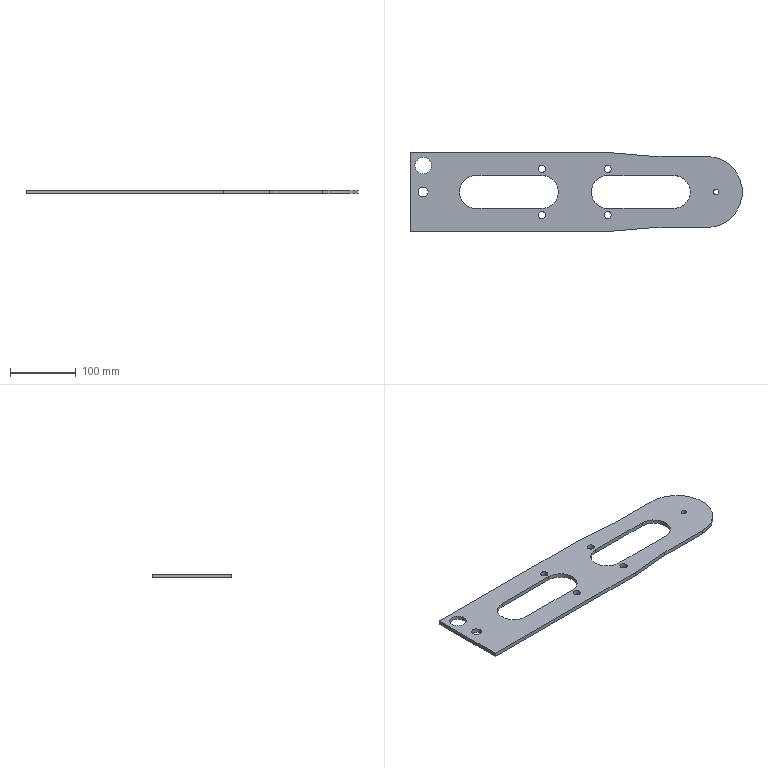Part | SolidWorks | features Extrusion 1, HoleWzd 1, ICE 1 | 1 solid | 34 faces | box 504 x 120 x 6 mm | volume 253053 mm3 | cylinder 21 | plane 13 | commonest cylinder face diameters 11 x8 50 x6 8 x2 15 x2 25 x2 108 x1
STEP:
#1=CARTESIAN_POINT('',(205.5,60.,6.));
#2=VERTEX_POINT('',#1);
#3=CARTESIAN_POINT('',(213.5,60.,6.));
#4=VERTEX_POINT('',#3);
#5=CARTESIAN_POINT('',(209.5,60.,6.));
#6=DIRECTION('',(0.,0.,1.));
#7=DIRECTION('',(1.,0.,0.));
#8=AXIS2_PLACEMENT_3D('',#5,#6,#7);
#9=CIRCLE('',#8,4.);
#10=EDGE_CURVE('',#2,#4,#9,.T.);
#11=ORIENTED_EDGE('',*,*,#10,.T.);
#12=CARTESIAN_POINT('',(213.5,60.,0.));
#13=VERTEX_POINT('',#12);
#14=CARTESIAN_POINT('',(213.5,60.,10.));
#15=DIRECTION('',(0.,0.,-1.));
#16=VECTOR('',#15,1000.);
#17=LINE('',#14,#16);
#18=EDGE_CURVE('',#4,#13,#17,.T.);
#19=ORIENTED_EDGE('',*,*,#18,.T.);
#20=CARTESIAN_POINT('',(205.5,60.,0.));
#21=VERTEX_POINT('',#20);
#22=CARTESIAN_POINT('',(209.5,60.,0.));
#23=DIRECTION('',(0.,0.,-1.));
#24=DIRECTION('',(-1.,0.,0.));
#25=AXIS2_PLACEMENT_3D('',#22,#23,#24);
#26=CIRCLE('',#25,4.);
#27=EDGE_CURVE('',#13,#21,#26,.T.);
#28=ORIENTED_EDGE('',*,*,#27,.T.);
#29=CARTESIAN_POINT('',(205.5,60.,10.));
#30=DIRECTION('',(0.,0.,-1.));
#31=VECTOR('',#30,1000.);
#32=LINE('',#29,#31);
#33=EDGE_CURVE('',#2,#21,#32,.T.);
#34=ORIENTED_EDGE('',*,*,#33,.F.);
#35=EDGE_LOOP('',(#11,#19,#28,#34));
#36=FACE_OUTER_BOUND('',#35,.T.);
#37=CARTESIAN_POINT('',(209.5,60.,10.));
#38=DIRECTION('',(0.,0.,-1.));
#39=DIRECTION('',(-1.,0.,0.));
#40=AXIS2_PLACEMENT_3D('',#37,#38,#39);
#41=CYLINDRICAL_SURFACE('',#40,4.);
#42=ADVANCED_FACE('',(#36),#41,.F.);
#43=CARTESIAN_POINT('',(-60.5,95.,0.));
#44=VERTEX_POINT('',#43);
#45=CARTESIAN_POINT('',(-49.5,95.,0.));
#46=VERTEX_POINT('',#45);
#47=CARTESIAN_POINT('',(-55.,95.,0.));
#48=DIRECTION('',(0.,0.,1.));
#49=DIRECTION('',(1.,0.,0.));
#50=AXIS2_PLACEMENT_3D('',#47,#48,#49);
#51=CIRCLE('',#50,5.5);
#52=EDGE_CURVE('',#44,#46,#51,.T.);
#53=ORIENTED_EDGE('',*,*,#52,.F.);
#54=CARTESIAN_POINT('',(-60.5,95.,6.));
#55=VERTEX_POINT('',#54);
#56=CARTESIAN_POINT('',(-60.5,95.,6.));
#57=DIRECTION('',(0.,0.,1.));
#58=VECTOR('',#57,1000.);
#59=LINE('',#56,#58);
#60=EDGE_CURVE('',#44,#55,#59,.T.);
#61=ORIENTED_EDGE('',*,*,#60,.T.);
#62=CARTESIAN_POINT('',(-49.5,95.,6.));
#63=VERTEX_POINT('',#62);
#64=CARTESIAN_POINT('',(-55.,95.,6.));
#65=DIRECTION('',(0.,0.,1.));
#66=DIRECTION('',(1.,0.,0.));
#67=AXIS2_PLACEMENT_3D('',#64,#65,#66);
#68=CIRCLE('',#67,5.5);
#69=EDGE_CURVE('',#55,#63,#68,.T.);
#70=ORIENTED_EDGE('',*,*,#69,.T.);
#71=CARTESIAN_POINT('',(-49.5,95.,6.));
#72=DIRECTION('',(0.,0.,1.));
#73=VECTOR('',#72,1000.);
#74=LINE('',#71,#73);
#75=EDGE_CURVE('',#46,#63,#74,.T.);
#76=ORIENTED_EDGE('',*,*,#75,.F.);
#77=EDGE_LOOP('',(#53,#61,#70,#76));
#78=FACE_OUTER_BOUND('',#77,.T.);
#79=CARTESIAN_POINT('',(-55.,95.,6.));
#80=DIRECTION('',(0.,0.,1.));
#81=DIRECTION('',(1.,0.,0.));
#82=AXIS2_PLACEMENT_3D('',#79,#80,#81);
#83=CYLINDRICAL_SURFACE('',#82,5.5);
#84=ADVANCED_FACE('',(#78),#83,.F.);
#85=CARTESIAN_POINT('',(-60.5,25.,0.));
#86=VERTEX_POINT('',#85);
#87=CARTESIAN_POINT('',(-49.5,25.,0.));
#88=VERTEX_POINT('',#87);
#89=CARTESIAN_POINT('',(-55.,25.,0.));
#90=DIRECTION('',(0.,0.,1.));
#91=DIRECTION('',(1.,0.,0.));
#92=AXIS2_PLACEMENT_3D('',#89,#90,#91);
#93=CIRCLE('',#92,5.5);
#94=EDGE_CURVE('',#86,#88,#93,.T.);
#95=ORIENTED_EDGE('',*,*,#94,.F.);
#96=CARTESIAN_POINT('',(-60.5,25.,6.));
#97=VERTEX_POINT('',#96);
#98=CARTESIAN_POINT('',(-60.5,25.,6.));
#99=DIRECTION('',(0.,0.,1.));
#100=VECTOR('',#99,1000.);
#101=LINE('',#98,#100);
#102=EDGE_CURVE('',#86,#97,#101,.T.);
#103=ORIENTED_EDGE('',*,*,#102,.T.);
#104=CARTESIAN_POINT('',(-49.5,25.,6.));
#105=VERTEX_POINT('',#104);
#106=CARTESIAN_POINT('',(-55.,25.,6.));
#107=DIRECTION('',(0.,0.,1.));
#108=DIRECTION('',(1.,0.,0.));
#109=AXIS2_PLACEMENT_3D('',#106,#107,#108);
#110=CIRCLE('',#109,5.5);
#111=EDGE_CURVE('',#97,#105,#110,.T.);
#112=ORIENTED_EDGE('',*,*,#111,.T.);
#113=CARTESIAN_POINT('',(-49.5,25.,6.));
#114=DIRECTION('',(0.,0.,1.));
#115=VECTOR('',#114,1000.);
#116=LINE('',#113,#115);
#117=EDGE_CURVE('',#88,#105,#116,.T.);
#118=ORIENTED_EDGE('',*,*,#117,.F.);
#119=EDGE_LOOP('',(#95,#103,#112,#118));
#120=FACE_OUTER_BOUND('',#119,.T.);
#121=CARTESIAN_POINT('',(-55.,25.,6.));
#122=DIRECTION('',(0.,0.,1.));
#123=DIRECTION('',(1.,0.,0.));
#124=AXIS2_PLACEMENT_3D('',#121,#122,#123);
#125=CYLINDRICAL_SURFACE('',#124,5.5);
#126=ADVANCED_FACE('',(#120),#125,.F.);
#127=CARTESIAN_POINT('',(39.5,95.,0.));
#128=VERTEX_POINT('',#127);
#129=CARTESIAN_POINT('',(50.5,95.,0.));
#130=VERTEX_POINT('',#129);
#131=CARTESIAN_POINT('',(45.,95.,0.));
#132=DIRECTION('',(0.,0.,1.));
#133=DIRECTION('',(1.,0.,0.));
#134=AXIS2_PLACEMENT_3D('',#131,#132,#133);
#135=CIRCLE('',#134,5.5);
#136=EDGE_CURVE('',#128,#130,#135,.T.);
#137=ORIENTED_EDGE('',*,*,#136,.F.);
#138=CARTESIAN_POINT('',(39.5,95.,6.));
#139=VERTEX_POINT('',#138);
#140=CARTESIAN_POINT('',(39.5,95.,6.));
#141=DIRECTION('',(0.,0.,1.));
#142=VECTOR('',#141,1000.);
#143=LINE('',#140,#142);
#144=EDGE_CURVE('',#128,#139,#143,.T.);
#145=ORIENTED_EDGE('',*,*,#144,.T.);
#146=CARTESIAN_POINT('',(50.5,95.,6.));
#147=VERTEX_POINT('',#146);
#148=CARTESIAN_POINT('',(45.,95.,6.));
#149=DIRECTION('',(0.,0.,1.));
#150=DIRECTION('',(1.,0.,0.));
#151=AXIS2_PLACEMENT_3D('',#148,#149,#150);
#152=CIRCLE('',#151,5.5);
#153=EDGE_CURVE('',#139,#147,#152,.T.);
#154=ORIENTED_EDGE('',*,*,#153,.T.);
#155=CARTESIAN_POINT('',(50.5,95.,6.));
#156=DIRECTION('',(0.,0.,1.));
#157=VECTOR('',#156,1000.);
#158=LINE('',#155,#157);
#159=EDGE_CURVE('',#130,#147,#158,.T.);
#160=ORIENTED_EDGE('',*,*,#159,.F.);
#161=EDGE_LOOP('',(#137,#145,#154,#160));
#162=FACE_OUTER_BOUND('',#161,.T.);
#163=CARTESIAN_POINT('',(45.,95.,6.));
#164=DIRECTION('',(0.,0.,1.));
#165=DIRECTION('',(1.,0.,0.));
#166=AXIS2_PLACEMENT_3D('',#163,#164,#165);
#167=CYLINDRICAL_SURFACE('',#166,5.5);
#168=ADVANCED_FACE('',(#162),#167,.F.);
#169=CARTESIAN_POINT('',(39.5,25.,0.));
#170=VERTEX_POINT('',#169);
#171=CARTESIAN_POINT('',(50.5,25.,0.));
#172=VERTEX_POINT('',#171);
#173=CARTESIAN_POINT('',(45.,25.,0.));
#174=DIRECTION('',(0.,0.,1.));
#175=DIRECTION('',(1.,0.,0.));
#176=AXIS2_PLACEMENT_3D('',#173,#174,#175);
#177=CIRCLE('',#176,5.5);
#178=EDGE_CURVE('',#170,#172,#177,.T.);
#179=ORIENTED_EDGE('',*,*,#178,.F.);
#180=CARTESIAN_POINT('',(39.5,25.,6.));
#181=VERTEX_POINT('',#180);
#182=CARTESIAN_POINT('',(39.5,25.,6.));
#183=DIRECTION('',(0.,0.,1.));
#184=VECTOR('',#183,1000.);
#185=LINE('',#182,#184);
#186=EDGE_CURVE('',#170,#181,#185,.T.);
#187=ORIENTED_EDGE('',*,*,#186,.T.);
#188=CARTESIAN_POINT('',(50.5,25.,6.));
#189=VERTEX_POINT('',#188);
#190=CARTESIAN_POINT('',(45.,25.,6.));
#191=DIRECTION('',(0.,0.,1.));
#192=DIRECTION('',(1.,0.,0.));
#193=AXIS2_PLACEMENT_3D('',#190,#191,#192);
#194=CIRCLE('',#193,5.5);
#195=EDGE_CURVE('',#181,#189,#194,.T.);
#196=ORIENTED_EDGE('',*,*,#195,.T.);
#197=CARTESIAN_POINT('',(50.5,25.,6.));
#198=DIRECTION('',(0.,0.,1.));
#199=VECTOR('',#198,1000.);
#200=LINE('',#197,#199);
#201=EDGE_CURVE('',#172,#189,#200,.T.);
#202=ORIENTED_EDGE('',*,*,#201,.F.);
#203=EDGE_LOOP('',(#179,#187,#196,#202));
#204=FACE_OUTER_BOUND('',#203,.T.);
#205=CARTESIAN_POINT('',(45.,25.,6.));
#206=DIRECTION('',(0.,0.,1.));
#207=DIRECTION('',(1.,0.,0.));
#208=AXIS2_PLACEMENT_3D('',#205,#206,#207);
#209=CYLINDRICAL_SURFACE('',#208,5.5);
#210=ADVANCED_FACE('',(#204),#209,.F.);
#211=CARTESIAN_POINT('',(45.,85.,6.));
#212=VERTEX_POINT('',#211);
#213=CARTESIAN_POINT('',(20.,60.,6.));
#214=VERTEX_POINT('',#213);
#215=CARTESIAN_POINT('',(45.,60.,6.));
#216=DIRECTION('',(0.,0.,1.));
#217=DIRECTION('',(1.,0.,0.));
#218=AXIS2_PLACEMENT_3D('',#215,#216,#217);
#219=CIRCLE('',#218,25.);
#220=EDGE_CURVE('',#212,#214,#219,.T.);
#221=ORIENTED_EDGE('',*,*,#220,.T.);
#222=CARTESIAN_POINT('',(20.,60.,0.));
#223=VERTEX_POINT('',#222);
#224=CARTESIAN_POINT('',(20.,60.,6.));
#225=DIRECTION('',(0.,0.,-1.));
#226=VECTOR('',#225,1000.);
#227=LINE('',#224,#226);
#228=EDGE_CURVE('',#214,#223,#227,.T.);
#229=ORIENTED_EDGE('',*,*,#228,.T.);
#230=CARTESIAN_POINT('',(45.,85.,0.));
#231=VERTEX_POINT('',#230);
#232=CARTESIAN_POINT('',(45.,60.,0.));
#233=DIRECTION('',(0.,0.,1.));
#234=DIRECTION('',(1.,0.,0.));
#235=AXIS2_PLACEMENT_3D('',#232,#233,#234);
#236=CIRCLE('',#235,25.);
#237=EDGE_CURVE('',#231,#223,#236,.T.);
#238=ORIENTED_EDGE('',*,*,#237,.F.);
#239=CARTESIAN_POINT('',(45.,85.,6.));
#240=DIRECTION('',(0.,0.,-1.));
#241=VECTOR('',#240,1000.);
#242=LINE('',#239,#241);
#243=EDGE_CURVE('',#212,#231,#242,.T.);
#244=ORIENTED_EDGE('',*,*,#243,.F.);
#245=EDGE_LOOP('',(#221,#229,#238,#244));
#246=FACE_OUTER_BOUND('',#245,.T.);
#247=CARTESIAN_POINT('',(45.,60.,6.));
#248=DIRECTION('',(0.,0.,-1.));
#249=DIRECTION('',(-1.,0.,0.));
#250=AXIS2_PLACEMENT_3D('',#247,#248,#249);
#251=CYLINDRICAL_SURFACE('',#250,25.);
#252=ADVANCED_FACE('',(#246),#251,.F.);
#253=CARTESIAN_POINT('',(-155.,85.,6.));
#254=VERTEX_POINT('',#253);
#255=CARTESIAN_POINT('',(-180.,60.,6.));
#256=VERTEX_POINT('',#255);
#257=CARTESIAN_POINT('',(-155.,60.,6.));
#258=DIRECTION('',(0.,0.,1.));
#259=DIRECTION('',(1.,0.,0.));
#260=AXIS2_PLACEMENT_3D('',#257,#258,#259);
#261=CIRCLE('',#260,25.);
#262=EDGE_CURVE('',#254,#256,#261,.T.);
#263=ORIENTED_EDGE('',*,*,#262,.T.);
#264=CARTESIAN_POINT('',(-180.,60.,0.));
#265=VERTEX_POINT('',#264);
#266=CARTESIAN_POINT('',(-180.,60.,6.));
#267=DIRECTION('',(0.,0.,-1.));
#268=VECTOR('',#267,1000.);
#269=LINE('',#266,#268);
#270=EDGE_CURVE('',#256,#265,#269,.T.);
#271=ORIENTED_EDGE('',*,*,#270,.T.);
#272=CARTESIAN_POINT('',(-155.,85.,0.));
#273=VERTEX_POINT('',#272);
#274=CARTESIAN_POINT('',(-155.,60.,0.));
#275=DIRECTION('',(0.,0.,1.));
#276=DIRECTION('',(1.,0.,0.));
#277=AXIS2_PLACEMENT_3D('',#274,#275,#276);
#278=CIRCLE('',#277,25.);
#279=EDGE_CURVE('',#273,#265,#278,.T.);
#280=ORIENTED_EDGE('',*,*,#279,.F.);
#281=CARTESIAN_POINT('',(-155.,85.,6.));
#282=DIRECTION('',(0.,0.,-1.));
#283=VECTOR('',#282,1000.);
#284=LINE('',#281,#283);
#285=EDGE_CURVE('',#254,#273,#284,.T.);
#286=ORIENTED_EDGE('',*,*,#285,.F.);
#287=EDGE_LOOP('',(#263,#271,#280,#286));
#288=FACE_OUTER_BOUND('',#287,.T.);
#289=CARTESIAN_POINT('',(-155.,60.,6.));
#290=DIRECTION('',(0.,0.,-1.));
#291=DIRECTION('',(-1.,0.,0.));
#292=AXIS2_PLACEMENT_3D('',#289,#290,#291);
#293=CYLINDRICAL_SURFACE('',#292,25.);
#294=ADVANCED_FACE('',(#288),#293,.F.);
#295=CARTESIAN_POINT('',(-242.5,60.,6.));
#296=VERTEX_POINT('',#295);
#297=CARTESIAN_POINT('',(-227.5,60.,6.));
#298=VERTEX_POINT('',#297);
#299=CARTESIAN_POINT('',(-235.,60.,6.));
#300=DIRECTION('',(0.,0.,1.));
#301=DIRECTION('',(1.,0.,0.));
#302=AXIS2_PLACEMENT_3D('',#299,#300,#301);
#303=CIRCLE('',#302,7.5);
#304=EDGE_CURVE('',#296,#298,#303,.T.);
#305=ORIENTED_EDGE('',*,*,#304,.T.);
#306=CARTESIAN_POINT('',(-227.5,60.,0.));
#307=VERTEX_POINT('',#306);
#308=CARTESIAN_POINT('',(-227.5,60.,6.));
#309=DIRECTION('',(0.,0.,-1.));
#310=VECTOR('',#309,1000.);
#311=LINE('',#308,#310);
#312=EDGE_CURVE('',#298,#307,#311,.T.);
#313=ORIENTED_EDGE('',*,*,#312,.T.);
#314=CARTESIAN_POINT('',(-242.5,60.,0.));
#315=VERTEX_POINT('',#314);
#316=CARTESIAN_POINT('',(-235.,60.,0.));
#317=DIRECTION('',(0.,0.,1.));
#318=DIRECTION('',(1.,0.,0.));
#319=AXIS2_PLACEMENT_3D('',#316,#317,#318);
#320=CIRCLE('',#319,7.5);
#321=EDGE_CURVE('',#315,#307,#320,.T.);
#322=ORIENTED_EDGE('',*,*,#321,.F.);
#323=CARTESIAN_POINT('',(-242.5,60.,6.));
#324=DIRECTION('',(0.,0.,-1.));
#325=VECTOR('',#324,1000.);
#326=LINE('',#323,#325);
#327=EDGE_CURVE('',#296,#315,#326,.T.);
#328=ORIENTED_EDGE('',*,*,#327,.F.);
#329=EDGE_LOOP('',(#305,#313,#322,#328));
#330=FACE_OUTER_BOUND('',#329,.T.);
#331=CARTESIAN_POINT('',(-235.,60.,6.));
#332=DIRECTION('',(0.,0.,-1.));
#333=DIRECTION('',(-1.,0.,0.));
#334=AXIS2_PLACEMENT_3D('',#331,#332,#333);
#335=CYLINDRICAL_SURFACE('',#334,7.5);
#336=ADVANCED_FACE('',(#330),#335,.F.);
#337=CARTESIAN_POINT('',(-247.5,100.,6.));
#338=VERTEX_POINT('',#337);
#339=CARTESIAN_POINT('',(-222.5,100.,6.));
#340=VERTEX_POINT('',#339);
#341=CARTESIAN_POINT('',(-235.,100.,6.));
#342=DIRECTION('',(0.,0.,1.));
#343=DIRECTION('',(1.,0.,0.));
#344=AXIS2_PLACEMENT_3D('',#341,#342,#343);
#345=CIRCLE('',#344,12.5);
#346=EDGE_CURVE('',#338,#340,#345,.T.);
#347=ORIENTED_EDGE('',*,*,#346,.T.);
#348=CARTESIAN_POINT('',(-222.5,100.,0.));
#349=VERTEX_POINT('',#348);
#350=CARTESIAN_POINT('',(-222.5,100.,6.));
#351=DIRECTION('',(0.,0.,-1.));
#352=VECTOR('',#351,1000.);
#353=LINE('',#350,#352);
#354=EDGE_CURVE('',#340,#349,#353,.T.);
#355=ORIENTED_EDGE('',*,*,#354,.T.);
#356=CARTESIAN_POINT('',(-247.5,100.,0.));
#357=VERTEX_POINT('',#356);
#358=CARTESIAN_POINT('',(-235.,100.,0.));
#359=DIRECTION('',(0.,0.,1.));
#360=DIRECTION('',(1.,0.,0.));
#361=AXIS2_PLACEMENT_3D('',#358,#359,#360);
#362=CIRCLE('',#361,12.5);
#363=EDGE_CURVE('',#357,#349,#362,.T.);
#364=ORIENTED_EDGE('',*,*,#363,.F.);
#365=CARTESIAN_POINT('',(-247.5,100.,6.));
#366=DIRECTION('',(0.,0.,-1.));
#367=VECTOR('',#366,1000.);
#368=LINE('',#365,#367);
#369=EDGE_CURVE('',#338,#357,#368,.T.);
#370=ORIENTED_EDGE('',*,*,#369,.F.);
#371=EDGE_LOOP('',(#347,#355,#364,#370));
#372=FACE_OUTER_BOUND('',#371,.T.);
#373=CARTESIAN_POINT('',(-235.,100.,6.));
#374=DIRECTION('',(0.,0.,-1.));
#375=DIRECTION('',(-1.,0.,0.));
#376=AXIS2_PLACEMENT_3D('',#373,#374,#375);
#377=CYLINDRICAL_SURFACE('',#376,12.5);
#378=ADVANCED_FACE('',(#372),#377,.F.);
#379=CARTESIAN_POINT('',(209.5,60.,0.));
#380=DIRECTION('',(0.,0.,-1.));
#381=DIRECTION('',(-1.,0.,0.));
#382=AXIS2_PLACEMENT_3D('',#379,#380,#381);
#383=CIRCLE('',#382,4.);
#384=EDGE_CURVE('',#21,#13,#383,.T.);
#385=ORIENTED_EDGE('',*,*,#384,.F.);
#386=ORIENTED_EDGE('',*,*,#27,.F.);
#387=EDGE_LOOP('',(#385,#386));
#388=FACE_BOUND('',#387,.T.);
#389=CARTESIAN_POINT('',(-55.,95.,0.));
#390=DIRECTION('',(0.,0.,1.));
#391=DIRECTION('',(1.,0.,0.));
#392=AXIS2_PLACEMENT_3D('',#389,#390,#391);
#393=CIRCLE('',#392,5.5);
#394=EDGE_CURVE('',#46,#44,#393,.T.);
#395=ORIENTED_EDGE('',*,*,#394,.T.);
#396=ORIENTED_EDGE('',*,*,#52,.T.);
#397=EDGE_LOOP('',(#395,#396));
#398=FACE_BOUND('',#397,.T.);
#399=CARTESIAN_POINT('',(-55.,25.,0.));
#400=DIRECTION('',(0.,0.,1.));
#401=DIRECTION('',(1.,0.,0.));
#402=AXIS2_PLACEMENT_3D('',#399,#400,#401);
#403=CIRCLE('',#402,5.5);
#404=EDGE_CURVE('',#88,#86,#403,.T.);
#405=ORIENTED_EDGE('',*,*,#404,.T.);
#406=ORIENTED_EDGE('',*,*,#94,.T.);
#407=EDGE_LOOP('',(#405,#406));
#408=FACE_BOUND('',#407,.T.);
#409=CARTESIAN_POINT('',(45.,95.,0.));
#410=DIRECTION('',(0.,0.,1.));
#411=DIRECTION('',(1.,0.,0.));
#412=AXIS2_PLACEMENT_3D('',#409,#410,#411);
#413=CIRCLE('',#412,5.5);
#414=EDGE_CURVE('',#130,#128,#413,.T.);
#415=ORIENTED_EDGE('',*,*,#414,.T.);
#416=ORIENTED_EDGE('',*,*,#136,.T.);
#417=EDGE_LOOP('',(#415,#416));
#418=FACE_BOUND('',#417,.T.);
#419=CARTESIAN_POINT('',(45.,25.,0.));
#420=DIRECTION('',(0.,0.,1.));
#421=DIRECTION('',(1.,0.,0.));
#422=AXIS2_PLACEMENT_3D('',#419,#420,#421);
#423=CIRCLE('',#422,5.5);
#424=EDGE_CURVE('',#172,#170,#423,.T.);
#425=ORIENTED_EDGE('',*,*,#424,.T.);
#426=ORIENTED_EDGE('',*,*,#178,.T.);
#427=EDGE_LOOP('',(#425,#426));
#428=FACE_BOUND('',#427,.T.);
#429=ORIENTED_EDGE('',*,*,#279,.T.);
#430=CARTESIAN_POINT('',(-155.,35.,0.));
#431=VERTEX_POINT('',#430);
#432=CARTESIAN_POINT('',(-155.,60.,0.));
#433=DIRECTION('',(0.,0.,1.));
#434=DIRECTION('',(1.,0.,0.));
#435=AXIS2_PLACEMENT_3D('',#432,#433,#434);
#436=CIRCLE('',#435,25.);
#437=EDGE_CURVE('',#265,#431,#436,.T.);
#438=ORIENTED_EDGE('',*,*,#437,.T.);
#439=CARTESIAN_POINT('',(-55.,35.,0.));
#440=VERTEX_POINT('',#439);
#441=CARTESIAN_POINT('',(-155.,35.,0.));
#442=DIRECTION('',(1.,0.,0.));
#443=VECTOR('',#442,1000.);
#444=LINE('',#441,#443);
#445=EDGE_CURVE('',#431,#440,#444,.T.);
#446=ORIENTED_EDGE('',*,*,#445,.T.);
#447=CARTESIAN_POINT('',(-55.,85.,0.));
#448=VERTEX_POINT('',#447);
#449=CARTESIAN_POINT('',(-55.,60.,0.));
#450=DIRECTION('',(0.,0.,1.));
#451=DIRECTION('',(1.,0.,0.));
#452=AXIS2_PLACEMENT_3D('',#449,#450,#451);
#453=CIRCLE('',#452,25.);
#454=EDGE_CURVE('',#440,#448,#453,.T.);
#455=ORIENTED_EDGE('',*,*,#454,.T.);
#456=CARTESIAN_POINT('',(-155.,85.,0.));
#457=DIRECTION('',(-1.,0.,0.));
#458=VECTOR('',#457,1000.);
#459=LINE('',#456,#458);
#460=EDGE_CURVE('',#448,#273,#459,.T.);
#461=ORIENTED_EDGE('',*,*,#460,.T.);
#462=EDGE_LOOP('',(#429,#438,#446,#455,#461));
#463=FACE_BOUND('',#462,.T.);
#464=CARTESIAN_POINT('',(-255.,120.,0.));
#465=VERTEX_POINT('',#464);
#466=CARTESIAN_POINT('',(-255.,0.,0.));
#467=VERTEX_POINT('',#466);
#468=CARTESIAN_POINT('',(-255.,0.,0.));
#469=DIRECTION('',(0.,-1.,0.));
#470=VECTOR('',#469,1000.);
#471=LINE('',#468,#470);
#472=EDGE_CURVE('',#465,#467,#471,.T.);
#473=ORIENTED_EDGE('',*,*,#472,.F.);
#474=CARTESIAN_POINT('',(45.,120.,0.));
#475=VERTEX_POINT('',#474);
#476=CARTESIAN_POINT('',(-255.,120.,0.));
#477=DIRECTION('',(-1.,0.,0.));
#478=VECTOR('',#477,1000.);
#479=LINE('',#476,#478);
#480=EDGE_CURVE('',#475,#465,#479,.T.);
#481=ORIENTED_EDGE('',*,*,#480,.F.);
#482=CARTESIAN_POINT('',(115.,114.,0.));
#483=VERTEX_POINT('',#482);
#484=CARTESIAN_POINT('',(45.,120.,0.));
#485=DIRECTION('',(-0.9963,0.0854,0.));
#486=VECTOR('',#485,1000.);
#487=LINE('',#484,#486);
#488=EDGE_CURVE('',#483,#475,#487,.T.);
#489=ORIENTED_EDGE('',*,*,#488,.F.);
#490=CARTESIAN_POINT('',(195.,114.,0.));
#491=VERTEX_POINT('',#490);
#492=CARTESIAN_POINT('',(115.,114.,0.));
#493=DIRECTION('',(-1.,0.,0.));
#494=VECTOR('',#493,1000.);
#495=LINE('',#492,#494);
#496=EDGE_CURVE('',#491,#483,#495,.T.);
#497=ORIENTED_EDGE('',*,*,#496,.F.);
#498=CARTESIAN_POINT('',(195.,6.,0.));
#499=VERTEX_POINT('',#498);
#500=CARTESIAN_POINT('',(195.,60.,0.));
#501=DIRECTION('',(0.,0.,1.));
#502=DIRECTION('',(1.,0.,0.));
#503=AXIS2_PLACEMENT_3D('',#500,#501,#502);
#504=CIRCLE('',#503,54.);
#505=EDGE_CURVE('',#499,#491,#504,.T.);
#506=ORIENTED_EDGE('',*,*,#505,.F.);
#507=CARTESIAN_POINT('',(115.,6.,0.));
#508=VERTEX_POINT('',#507);
#509=CARTESIAN_POINT('',(115.,6.,0.));
#510=DIRECTION('',(1.,0.,0.));
#511=VECTOR('',#510,1000.);
#512=LINE('',#509,#511);
#513=EDGE_CURVE('',#508,#499,#512,.T.);
#514=ORIENTED_EDGE('',*,*,#513,.F.);
#515=CARTESIAN_POINT('',(45.,0.,0.));
#516=VERTEX_POINT('',#515);
#517=CARTESIAN_POINT('',(45.,0.,0.));
#518=DIRECTION('',(0.9963,0.0854,0.));
#519=VECTOR('',#518,1000.);
#520=LINE('',#517,#519);
#521=EDGE_CURVE('',#516,#508,#520,.T.);
#522=ORIENTED_EDGE('',*,*,#521,.F.);
#523=CARTESIAN_POINT('',(-255.,0.,0.));
#524=DIRECTION('',(1.,0.,0.));
#525=VECTOR('',#524,1000.);
#526=LINE('',#523,#525);
#527=EDGE_CURVE('',#467,#516,#526,.T.);
#528=ORIENTED_EDGE('',*,*,#527,.F.);
#529=EDGE_LOOP('',(#473,#481,#489,#497,#506,#514,#522,#528));
#530=FACE_OUTER_BOUND('',#529,.T.);
#531=ORIENTED_EDGE('',*,*,#363,.T.);
#532=CARTESIAN_POINT('',(-235.,100.,0.));
#533=DIRECTION('',(0.,0.,1.));
#534=DIRECTION('',(1.,0.,0.));
#535=AXIS2_PLACEMENT_3D('',#532,#533,#534);
#536=CIRCLE('',#535,12.5);
#537=EDGE_CURVE('',#349,#357,#536,.T.);
#538=ORIENTED_EDGE('',*,*,#537,.T.);
#539=EDGE_LOOP('',(#531,#538));
#540=FACE_BOUND('',#539,.T.);
#541=ORIENTED_EDGE('',*,*,#321,.T.);
#542=CARTESIAN_POINT('',(-235.,60.,0.));
#543=DIRECTION('',(0.,0.,1.));
#544=DIRECTION('',(1.,0.,0.));
#545=AXIS2_PLACEMENT_3D('',#542,#543,#544);
#546=CIRCLE('',#545,7.5);
#547=EDGE_CURVE('',#307,#315,#546,.T.);
#548=ORIENTED_EDGE('',*,*,#547,.T.);
#549=EDGE_LOOP('',(#541,#548));
#550=FACE_BOUND('',#549,.T.);
#551=ORIENTED_EDGE('',*,*,#237,.T.);
#552=CARTESIAN_POINT('',(45.,35.,0.));
#553=VERTEX_POINT('',#552);
#554=CARTESIAN_POINT('',(45.,60.,0.));
#555=DIRECTION('',(0.,0.,1.));
#556=DIRECTION('',(1.,0.,0.));
#557=AXIS2_PLACEMENT_3D('',#554,#555,#556);
#558=CIRCLE('',#557,25.);
#559=EDGE_CURVE('',#223,#553,#558,.T.);
#560=ORIENTED_EDGE('',*,*,#559,.T.);
#561=CARTESIAN_POINT('',(145.,35.,0.));
#562=VERTEX_POINT('',#561);
#563=CARTESIAN_POINT('',(45.,35.,0.));
#564=DIRECTION('',(1.,0.,0.));
#565=VECTOR('',#564,1000.);
#566=LINE('',#563,#565);
#567=EDGE_CURVE('',#553,#562,#566,.T.);
#568=ORIENTED_EDGE('',*,*,#567,.T.);
#569=CARTESIAN_POINT('',(145.,85.,0.));
#570=VERTEX_POINT('',#569);
#571=CARTESIAN_POINT('',(145.,60.,0.));
#572=DIRECTION('',(0.,0.,1.));
#573=DIRECTION('',(1.,0.,0.));
#574=AXIS2_PLACEMENT_3D('',#571,#572,#573);
#575=CIRCLE('',#574,25.);
#576=EDGE_CURVE('',#562,#570,#575,.T.);
#577=ORIENTED_EDGE('',*,*,#576,.T.);
#578=CARTESIAN_POINT('',(45.,85.,0.));
#579=DIRECTION('',(-1.,0.,0.));
#580=VECTOR('',#579,1000.);
#581=LINE('',#578,#580);
#582=EDGE_CURVE('',#570,#231,#581,.T.);
#583=ORIENTED_EDGE('',*,*,#582,.T.);
#584=EDGE_LOOP('',(#551,#560,#568,#577,#583));
#585=FACE_BOUND('',#584,.T.);
#586=CARTESIAN_POINT('',(195.,60.,0.));
#587=DIRECTION('',(0.,0.,1.));
#588=DIRECTION('',(1.,0.,0.));
#589=AXIS2_PLACEMENT_3D('',#586,#587,#588);
#590=PLANE('',#589);
#591=ADVANCED_FACE('',(#388,#398,#408,#418,#428,#463,#530,#540,#550,#585),#590,.F.);
#592=ORIENTED_EDGE('',*,*,#10,.F.);
#593=CARTESIAN_POINT('',(209.5,60.,6.));
#594=DIRECTION('',(0.,0.,1.));
#595=DIRECTION('',(1.,0.,0.));
#596=AXIS2_PLACEMENT_3D('',#593,#594,#595);
#597=CIRCLE('',#596,4.);
#598=EDGE_CURVE('',#4,#2,#597,.T.);
#599=ORIENTED_EDGE('',*,*,#598,.F.);
#600=EDGE_LOOP('',(#592,#599));
#601=FACE_BOUND('',#600,.T.);
#602=CARTESIAN_POINT('',(-55.,95.,6.));
#603=DIRECTION('',(0.,0.,1.));
#604=DIRECTION('',(1.,0.,0.));
#605=AXIS2_PLACEMENT_3D('',#602,#603,#604);
#606=CIRCLE('',#605,5.5);
#607=EDGE_CURVE('',#63,#55,#606,.T.);
#608=ORIENTED_EDGE('',*,*,#607,.F.);
#609=ORIENTED_EDGE('',*,*,#69,.F.);
#610=EDGE_LOOP('',(#608,#609));
#611=FACE_BOUND('',#610,.T.);
#612=CARTESIAN_POINT('',(-55.,25.,6.));
#613=DIRECTION('',(0.,0.,1.));
#614=DIRECTION('',(1.,0.,0.));
#615=AXIS2_PLACEMENT_3D('',#612,#613,#614);
#616=CIRCLE('',#615,5.5);
#617=EDGE_CURVE('',#105,#97,#616,.T.);
#618=ORIENTED_EDGE('',*,*,#617,.F.);
#619=ORIENTED_EDGE('',*,*,#111,.F.);
#620=EDGE_LOOP('',(#618,#619));
#621=FACE_BOUND('',#620,.T.);
#622=CARTESIAN_POINT('',(45.,95.,6.));
#623=DIRECTION('',(0.,0.,1.));
#624=DIRECTION('',(1.,0.,0.));
#625=AXIS2_PLACEMENT_3D('',#622,#623,#624);
#626=CIRCLE('',#625,5.5);
#627=EDGE_CURVE('',#147,#139,#626,.T.);
#628=ORIENTED_EDGE('',*,*,#627,.F.);
#629=ORIENTED_EDGE('',*,*,#153,.F.);
#630=EDGE_LOOP('',(#628,#629));
#631=FACE_BOUND('',#630,.T.);
#632=CARTESIAN_POINT('',(45.,25.,6.));
#633=DIRECTION('',(0.,0.,1.));
#634=DIRECTION('',(1.,0.,0.));
#635=AXIS2_PLACEMENT_3D('',#632,#633,#634);
#636=CIRCLE('',#635,5.5);
#637=EDGE_CURVE('',#189,#181,#636,.T.);
#638=ORIENTED_EDGE('',*,*,#637,.F.);
#639=ORIENTED_EDGE('',*,*,#195,.F.);
#640=EDGE_LOOP('',(#638,#639));
#641=FACE_BOUND('',#640,.T.);
#642=ORIENTED_EDGE('',*,*,#346,.F.);
#643=CARTESIAN_POINT('',(-235.,100.,6.));
#644=DIRECTION('',(0.,0.,1.));
#645=DIRECTION('',(1.,0.,0.));
#646=AXIS2_PLACEMENT_3D('',#643,#644,#645);
#647=CIRCLE('',#646,12.5);
#648=EDGE_CURVE('',#340,#338,#647,.T.);
#649=ORIENTED_EDGE('',*,*,#648,.F.);
#650=EDGE_LOOP('',(#642,#649));
#651=FACE_BOUND('',#650,.T.);
#652=CARTESIAN_POINT('',(-255.,120.,6.));
#653=VERTEX_POINT('',#652);
#654=CARTESIAN_POINT('',(-255.,0.,6.));
#655=VERTEX_POINT('',#654);
#656=CARTESIAN_POINT('',(-255.,0.,6.));
#657=DIRECTION('',(0.,-1.,0.));
#658=VECTOR('',#657,1000.);
#659=LINE('',#656,#658);
#660=EDGE_CURVE('',#653,#655,#659,.T.);
#661=ORIENTED_EDGE('',*,*,#660,.T.);
#662=CARTESIAN_POINT('',(45.,0.,6.));
#663=VERTEX_POINT('',#662);
#664=CARTESIAN_POINT('',(-255.,0.,6.));
#665=DIRECTION('',(1.,0.,0.));
#666=VECTOR('',#665,1000.);
#667=LINE('',#664,#666);
#668=EDGE_CURVE('',#655,#663,#667,.T.);
#669=ORIENTED_EDGE('',*,*,#668,.T.);
#670=CARTESIAN_POINT('',(115.,6.,6.));
#671=VERTEX_POINT('',#670);
#672=CARTESIAN_POINT('',(45.,0.,6.));
#673=DIRECTION('',(0.9963,0.0854,0.));
#674=VECTOR('',#673,1000.);
#675=LINE('',#672,#674);
#676=EDGE_CURVE('',#663,#671,#675,.T.);
#677=ORIENTED_EDGE('',*,*,#676,.T.);
#678=CARTESIAN_POINT('',(195.,6.,6.));
#679=VERTEX_POINT('',#678);
#680=CARTESIAN_POINT('',(115.,6.,6.));
#681=DIRECTION('',(1.,0.,0.));
#682=VECTOR('',#681,1000.);
#683=LINE('',#680,#682);
#684=EDGE_CURVE('',#671,#679,#683,.T.);
#685=ORIENTED_EDGE('',*,*,#684,.T.);
#686=CARTESIAN_POINT('',(195.,114.,6.));
#687=VERTEX_POINT('',#686);
#688=CARTESIAN_POINT('',(195.,60.,6.));
#689=DIRECTION('',(0.,0.,1.));
#690=DIRECTION('',(1.,0.,0.));
#691=AXIS2_PLACEMENT_3D('',#688,#689,#690);
#692=CIRCLE('',#691,54.);
#693=EDGE_CURVE('',#679,#687,#692,.T.);
#694=ORIENTED_EDGE('',*,*,#693,.T.);
#695=CARTESIAN_POINT('',(115.,114.,6.));
#696=VERTEX_POINT('',#695);
#697=CARTESIAN_POINT('',(115.,114.,6.));
#698=DIRECTION('',(-1.,0.,0.));
#699=VECTOR('',#698,1000.);
#700=LINE('',#697,#699);
#701=EDGE_CURVE('',#687,#696,#700,.T.);
#702=ORIENTED_EDGE('',*,*,#701,.T.);
#703=CARTESIAN_POINT('',(45.,120.,6.));
#704=VERTEX_POINT('',#703);
#705=CARTESIAN_POINT('',(45.,120.,6.));
#706=DIRECTION('',(-0.9963,0.0854,0.));
#707=VECTOR('',#706,1000.);
#708=LINE('',#705,#707);
#709=EDGE_CURVE('',#696,#704,#708,.T.);
#710=ORIENTED_EDGE('',*,*,#709,.T.);
#711=CARTESIAN_POINT('',(-235.,120.,6.));
#712=DIRECTION('',(-1.,0.,0.));
#713=VECTOR('',#712,1000.);
#714=LINE('',#711,#713);
#715=EDGE_CURVE('',#704,#653,#714,.T.);
#716=ORIENTED_EDGE('',*,*,#715,.T.);
#717=EDGE_LOOP('',(#661,#669,#677,#685,#694,#702,#710,#716));
#718=FACE_OUTER_BOUND('',#717,.T.);
#719=ORIENTED_EDGE('',*,*,#304,.F.);
#720=CARTESIAN_POINT('',(-235.,60.,6.));
#721=DIRECTION('',(0.,0.,1.));
#722=DIRECTION('',(1.,0.,0.));
#723=AXIS2_PLACEMENT_3D('',#720,#721,#722);
#724=CIRCLE('',#723,7.5);
#725=EDGE_CURVE('',#298,#296,#724,.T.);
#726=ORIENTED_EDGE('',*,*,#725,.F.);
#727=EDGE_LOOP('',(#719,#726));
#728=FACE_BOUND('',#727,.T.);
#729=CARTESIAN_POINT('',(-155.,35.,6.));
#730=VERTEX_POINT('',#729);
#731=CARTESIAN_POINT('',(-55.,35.,6.));
#732=VERTEX_POINT('',#731);
#733=CARTESIAN_POINT('',(-155.,35.,6.));
#734=DIRECTION('',(1.,0.,0.));
#735=VECTOR('',#734,1000.);
#736=LINE('',#733,#735);
#737=EDGE_CURVE('',#730,#732,#736,.T.);
#738=ORIENTED_EDGE('',*,*,#737,.F.);
#739=CARTESIAN_POINT('',(-155.,60.,6.));
#740=DIRECTION('',(0.,0.,1.));
#741=DIRECTION('',(1.,0.,0.));
#742=AXIS2_PLACEMENT_3D('',#739,#740,#741);
#743=CIRCLE('',#742,25.);
#744=EDGE_CURVE('',#256,#730,#743,.T.);
#745=ORIENTED_EDGE('',*,*,#744,.F.);
#746=ORIENTED_EDGE('',*,*,#262,.F.);
#747=CARTESIAN_POINT('',(-55.,85.,6.));
#748=VERTEX_POINT('',#747);
#749=CARTESIAN_POINT('',(-155.,85.,6.));
#750=DIRECTION('',(-1.,0.,0.));
#751=VECTOR('',#750,1000.);
#752=LINE('',#749,#751);
#753=EDGE_CURVE('',#748,#254,#752,.T.);
#754=ORIENTED_EDGE('',*,*,#753,.F.);
#755=CARTESIAN_POINT('',(-55.,60.,6.));
#756=DIRECTION('',(0.,0.,1.));
#757=DIRECTION('',(1.,0.,0.));
#758=AXIS2_PLACEMENT_3D('',#755,#756,#757);
#759=CIRCLE('',#758,25.);
#760=EDGE_CURVE('',#732,#748,#759,.T.);
#761=ORIENTED_EDGE('',*,*,#760,.F.);
#762=EDGE_LOOP('',(#738,#745,#746,#754,#761));
#763=FACE_BOUND('',#762,.T.);
#764=CARTESIAN_POINT('',(45.,35.,6.));
#765=VERTEX_POINT('',#764);
#766=CARTESIAN_POINT('',(145.,35.,6.));
#767=VERTEX_POINT('',#766);
#768=CARTESIAN_POINT('',(45.,35.,6.));
#769=DIRECTION('',(1.,0.,0.));
#770=VECTOR('',#769,1000.);
#771=LINE('',#768,#770);
#772=EDGE_CURVE('',#765,#767,#771,.T.);
#773=ORIENTED_EDGE('',*,*,#772,.F.);
#774=CARTESIAN_POINT('',(45.,60.,6.));
#775=DIRECTION('',(0.,0.,1.));
#776=DIRECTION('',(1.,0.,0.));
#777=AXIS2_PLACEMENT_3D('',#774,#775,#776);
#778=CIRCLE('',#777,25.);
#779=EDGE_CURVE('',#214,#765,#778,.T.);
#780=ORIENTED_EDGE('',*,*,#779,.F.);
#781=ORIENTED_EDGE('',*,*,#220,.F.);
#782=CARTESIAN_POINT('',(145.,85.,6.));
#783=VERTEX_POINT('',#782);
#784=CARTESIAN_POINT('',(45.,85.,6.));
#785=DIRECTION('',(-1.,0.,0.));
#786=VECTOR('',#785,1000.);
#787=LINE('',#784,#786);
#788=EDGE_CURVE('',#783,#212,#787,.T.);
#789=ORIENTED_EDGE('',*,*,#788,.F.);
#790=CARTESIAN_POINT('',(145.,60.,6.));
#791=DIRECTION('',(0.,0.,1.));
#792=DIRECTION('',(1.,0.,0.));
#793=AXIS2_PLACEMENT_3D('',#790,#791,#792);
#794=CIRCLE('',#793,25.);
#795=EDGE_CURVE('',#767,#783,#794,.T.);
#796=ORIENTED_EDGE('',*,*,#795,.F.);
#797=EDGE_LOOP('',(#773,#780,#781,#789,#796));
#798=FACE_BOUND('',#797,.T.);
#799=CARTESIAN_POINT('',(195.,60.,6.));
#800=DIRECTION('',(0.,0.,1.));
#801=DIRECTION('',(1.,0.,0.));
#802=AXIS2_PLACEMENT_3D('',#799,#800,#801);
#803=PLANE('',#802);
#804=ADVANCED_FACE('',(#601,#611,#621,#631,#641,#651,#718,#728,#763,#798),#803,.T.);
#805=ORIENTED_EDGE('',*,*,#472,.T.);
#806=CARTESIAN_POINT('',(-255.,0.,6.));
#807=DIRECTION('',(0.,0.,-1.));
#808=VECTOR('',#807,1000.);
#809=LINE('',#806,#808);
#810=EDGE_CURVE('',#655,#467,#809,.T.);
#811=ORIENTED_EDGE('',*,*,#810,.F.);
#812=ORIENTED_EDGE('',*,*,#660,.F.);
#813=CARTESIAN_POINT('',(-255.,120.,6.));
#814=DIRECTION('',(0.,0.,-1.));
#815=VECTOR('',#814,1000.);
#816=LINE('',#813,#815);
#817=EDGE_CURVE('',#653,#465,#816,.T.);
#818=ORIENTED_EDGE('',*,*,#817,.T.);
#819=EDGE_LOOP('',(#805,#811,#812,#818));
#820=FACE_OUTER_BOUND('',#819,.T.);
#821=CARTESIAN_POINT('',(-255.,0.,6.));
#822=DIRECTION('',(1.,0.,0.));
#823=DIRECTION('',(0.,0.,-1.));
#824=AXIS2_PLACEMENT_3D('',#821,#822,#823);
#825=PLANE('',#824);
#826=ADVANCED_FACE('',(#820),#825,.F.);
#827=ORIENTED_EDGE('',*,*,#527,.T.);
#828=CARTESIAN_POINT('',(45.,0.,6.));
#829=DIRECTION('',(0.,0.,-1.));
#830=VECTOR('',#829,1000.);
#831=LINE('',#828,#830);
#832=EDGE_CURVE('',#663,#516,#831,.T.);
#833=ORIENTED_EDGE('',*,*,#832,.F.);
#834=ORIENTED_EDGE('',*,*,#668,.F.);
#835=ORIENTED_EDGE('',*,*,#810,.T.);
#836=EDGE_LOOP('',(#827,#833,#834,#835));
#837=FACE_OUTER_BOUND('',#836,.T.);
#838=CARTESIAN_POINT('',(-255.,0.,6.));
#839=DIRECTION('',(0.,1.,0.));
#840=DIRECTION('',(0.,0.,1.));
#841=AXIS2_PLACEMENT_3D('',#838,#839,#840);
#842=PLANE('',#841);
#843=ADVANCED_FACE('',(#837),#842,.F.);
#844=ORIENTED_EDGE('',*,*,#521,.T.);
#845=CARTESIAN_POINT('',(115.,6.,6.));
#846=DIRECTION('',(0.,0.,-1.));
#847=VECTOR('',#846,1000.);
#848=LINE('',#845,#847);
#849=EDGE_CURVE('',#671,#508,#848,.T.);
#850=ORIENTED_EDGE('',*,*,#849,.F.);
#851=ORIENTED_EDGE('',*,*,#676,.F.);
#852=ORIENTED_EDGE('',*,*,#832,.T.);
#853=EDGE_LOOP('',(#844,#850,#851,#852));
#854=FACE_OUTER_BOUND('',#853,.T.);
#855=CARTESIAN_POINT('',(45.,0.,6.));
#856=DIRECTION('',(-0.0854,0.9963,0.));
#857=DIRECTION('',(-0.9963,-0.0854,0.));
#858=AXIS2_PLACEMENT_3D('',#855,#856,#857);
#859=PLANE('',#858);
#860=ADVANCED_FACE('',(#854),#859,.F.);
#861=ORIENTED_EDGE('',*,*,#513,.T.);
#862=CARTESIAN_POINT('',(195.,6.,6.));
#863=DIRECTION('',(0.,0.,-1.));
#864=VECTOR('',#863,1000.);
#865=LINE('',#862,#864);
#866=EDGE_CURVE('',#679,#499,#865,.T.);
#867=ORIENTED_EDGE('',*,*,#866,.F.);
#868=ORIENTED_EDGE('',*,*,#684,.F.);
#869=ORIENTED_EDGE('',*,*,#849,.T.);
#870=EDGE_LOOP('',(#861,#867,#868,#869));
#871=FACE_OUTER_BOUND('',#870,.T.);
#872=CARTESIAN_POINT('',(115.,6.,6.));
#873=DIRECTION('',(0.,1.,0.));
#874=DIRECTION('',(-1.,0.,0.));
#875=AXIS2_PLACEMENT_3D('',#872,#873,#874);
#876=PLANE('',#875);
#877=ADVANCED_FACE('',(#871),#876,.F.);
#878=ORIENTED_EDGE('',*,*,#505,.T.);
#879=CARTESIAN_POINT('',(195.,114.,6.));
#880=DIRECTION('',(0.,0.,-1.));
#881=VECTOR('',#880,1000.);
#882=LINE('',#879,#881);
#883=EDGE_CURVE('',#687,#491,#882,.T.);
#884=ORIENTED_EDGE('',*,*,#883,.F.);
#885=ORIENTED_EDGE('',*,*,#693,.F.);
#886=ORIENTED_EDGE('',*,*,#866,.T.);
#887=EDGE_LOOP('',(#878,#884,#885,#886));
#888=FACE_OUTER_BOUND('',#887,.T.);
#889=CARTESIAN_POINT('',(195.,60.,6.));
#890=DIRECTION('',(0.,0.,-1.));
#891=DIRECTION('',(-1.,0.,0.));
#892=AXIS2_PLACEMENT_3D('',#889,#890,#891);
#893=CYLINDRICAL_SURFACE('',#892,54.);
#894=ADVANCED_FACE('',(#888),#893,.T.);
#895=ORIENTED_EDGE('',*,*,#496,.T.);
#896=CARTESIAN_POINT('',(115.,114.,6.));
#897=DIRECTION('',(0.,0.,-1.));
#898=VECTOR('',#897,1000.);
#899=LINE('',#896,#898);
#900=EDGE_CURVE('',#696,#483,#899,.T.);
#901=ORIENTED_EDGE('',*,*,#900,.F.);
#902=ORIENTED_EDGE('',*,*,#701,.F.);
#903=ORIENTED_EDGE('',*,*,#883,.T.);
#904=EDGE_LOOP('',(#895,#901,#902,#903));
#905=FACE_OUTER_BOUND('',#904,.T.);
#906=CARTESIAN_POINT('',(115.,114.,6.));
#907=DIRECTION('',(0.,-1.,0.));
#908=DIRECTION('',(0.,0.,-1.));
#909=AXIS2_PLACEMENT_3D('',#906,#907,#908);
#910=PLANE('',#909);
#911=ADVANCED_FACE('',(#905),#910,.F.);
#912=ORIENTED_EDGE('',*,*,#488,.T.);
#913=CARTESIAN_POINT('',(45.,120.,6.));
#914=DIRECTION('',(0.,0.,-1.));
#915=VECTOR('',#914,1000.);
#916=LINE('',#913,#915);
#917=EDGE_CURVE('',#704,#475,#916,.T.);
#918=ORIENTED_EDGE('',*,*,#917,.F.);
#919=ORIENTED_EDGE('',*,*,#709,.F.);
#920=ORIENTED_EDGE('',*,*,#900,.T.);
#921=EDGE_LOOP('',(#912,#918,#919,#920));
#922=FACE_OUTER_BOUND('',#921,.T.);
#923=CARTESIAN_POINT('',(45.,120.,6.));
#924=DIRECTION('',(-0.0854,-0.9963,0.));
#925=DIRECTION('',(0.9963,-0.0854,0.));
#926=AXIS2_PLACEMENT_3D('',#923,#924,#925);
#927=PLANE('',#926);
#928=ADVANCED_FACE('',(#922),#927,.F.);
#929=ORIENTED_EDGE('',*,*,#480,.T.);
#930=ORIENTED_EDGE('',*,*,#817,.F.);
#931=ORIENTED_EDGE('',*,*,#715,.F.);
#932=ORIENTED_EDGE('',*,*,#917,.T.);
#933=EDGE_LOOP('',(#929,#930,#931,#932));
#934=FACE_OUTER_BOUND('',#933,.T.);
#935=CARTESIAN_POINT('',(-255.,120.,6.));
#936=DIRECTION('',(0.,-1.,0.));
#937=DIRECTION('',(0.,0.,-1.));
#938=AXIS2_PLACEMENT_3D('',#935,#936,#937);
#939=PLANE('',#938);
#940=ADVANCED_FACE('',(#934),#939,.F.);
#941=ORIENTED_EDGE('',*,*,#354,.F.);
#942=ORIENTED_EDGE('',*,*,#648,.T.);
#943=ORIENTED_EDGE('',*,*,#369,.T.);
#944=ORIENTED_EDGE('',*,*,#537,.F.);
#945=EDGE_LOOP('',(#941,#942,#943,#944));
#946=FACE_OUTER_BOUND('',#945,.T.);
#947=CARTESIAN_POINT('',(-235.,100.,6.));
#948=DIRECTION('',(0.,0.,-1.));
#949=DIRECTION('',(-1.,0.,0.));
#950=AXIS2_PLACEMENT_3D('',#947,#948,#949);
#951=CYLINDRICAL_SURFACE('',#950,12.5);
#952=ADVANCED_FACE('',(#946),#951,.F.);
#953=ORIENTED_EDGE('',*,*,#312,.F.);
#954=ORIENTED_EDGE('',*,*,#725,.T.);
#955=ORIENTED_EDGE('',*,*,#327,.T.);
#956=ORIENTED_EDGE('',*,*,#547,.F.);
#957=EDGE_LOOP('',(#953,#954,#955,#956));
#958=FACE_OUTER_BOUND('',#957,.T.);
#959=CARTESIAN_POINT('',(-235.,60.,6.));
#960=DIRECTION('',(0.,0.,-1.));
#961=DIRECTION('',(-1.,0.,0.));
#962=AXIS2_PLACEMENT_3D('',#959,#960,#961);
#963=CYLINDRICAL_SURFACE('',#962,7.5);
#964=ADVANCED_FACE('',(#958),#963,.F.);
#965=ORIENTED_EDGE('',*,*,#270,.F.);
#966=ORIENTED_EDGE('',*,*,#744,.T.);
#967=CARTESIAN_POINT('',(-155.,35.,6.));
#968=DIRECTION('',(0.,0.,-1.));
#969=VECTOR('',#968,1000.);
#970=LINE('',#967,#969);
#971=EDGE_CURVE('',#730,#431,#970,.T.);
#972=ORIENTED_EDGE('',*,*,#971,.T.);
#973=ORIENTED_EDGE('',*,*,#437,.F.);
#974=EDGE_LOOP('',(#965,#966,#972,#973));
#975=FACE_OUTER_BOUND('',#974,.T.);
#976=CARTESIAN_POINT('',(-155.,60.,6.));
#977=DIRECTION('',(0.,0.,-1.));
#978=DIRECTION('',(-1.,0.,0.));
#979=AXIS2_PLACEMENT_3D('',#976,#977,#978);
#980=CYLINDRICAL_SURFACE('',#979,25.);
#981=ADVANCED_FACE('',(#975),#980,.F.);
#982=ORIENTED_EDGE('',*,*,#445,.F.);
#983=ORIENTED_EDGE('',*,*,#971,.F.);
#984=ORIENTED_EDGE('',*,*,#737,.T.);
#985=CARTESIAN_POINT('',(-55.,35.,6.));
#986=DIRECTION('',(0.,0.,-1.));
#987=VECTOR('',#986,1000.);
#988=LINE('',#985,#987);
#989=EDGE_CURVE('',#732,#440,#988,.T.);
#990=ORIENTED_EDGE('',*,*,#989,.T.);
#991=EDGE_LOOP('',(#982,#983,#984,#990));
#992=FACE_OUTER_BOUND('',#991,.T.);
#993=CARTESIAN_POINT('',(-155.,35.,6.));
#994=DIRECTION('',(0.,1.,0.));
#995=DIRECTION('',(-1.,0.,0.));
#996=AXIS2_PLACEMENT_3D('',#993,#994,#995);
#997=PLANE('',#996);
#998=ADVANCED_FACE('',(#992),#997,.T.);
#999=ORIENTED_EDGE('',*,*,#454,.F.);
#1000=ORIENTED_EDGE('',*,*,#989,.F.);
#1001=ORIENTED_EDGE('',*,*,#760,.T.);
#1002=CARTESIAN_POINT('',(-55.,85.,6.));
#1003=DIRECTION('',(0.,0.,-1.));
#1004=VECTOR('',#1003,1000.);
#1005=LINE('',#1002,#1004);
#1006=EDGE_CURVE('',#748,#448,#1005,.T.);
#1007=ORIENTED_EDGE('',*,*,#1006,.T.);
#1008=EDGE_LOOP('',(#999,#1000,#1001,#1007));
#1009=FACE_OUTER_BOUND('',#1008,.T.);
#1010=CARTESIAN_POINT('',(-55.,60.,6.));
#1011=DIRECTION('',(0.,0.,-1.));
#1012=DIRECTION('',(-1.,0.,0.));
#1013=AXIS2_PLACEMENT_3D('',#1010,#1011,#1012);
#1014=CYLINDRICAL_SURFACE('',#1013,25.);
#1015=ADVANCED_FACE('',(#1009),#1014,.F.);
#1016=ORIENTED_EDGE('',*,*,#460,.F.);
#1017=ORIENTED_EDGE('',*,*,#1006,.F.);
#1018=ORIENTED_EDGE('',*,*,#753,.T.);
#1019=ORIENTED_EDGE('',*,*,#285,.T.);
#1020=EDGE_LOOP('',(#1016,#1017,#1018,#1019));
#1021=FACE_OUTER_BOUND('',#1020,.T.);
#1022=CARTESIAN_POINT('',(-155.,85.,6.));
#1023=DIRECTION('',(0.,-1.,0.));
#1024=DIRECTION('',(0.,0.,-1.));
#1025=AXIS2_PLACEMENT_3D('',#1022,#1023,#1024);
#1026=PLANE('',#1025);
#1027=ADVANCED_FACE('',(#1021),#1026,.T.);
#1028=ORIENTED_EDGE('',*,*,#228,.F.);
#1029=ORIENTED_EDGE('',*,*,#779,.T.);
#1030=CARTESIAN_POINT('',(45.,35.,6.));
#1031=DIRECTION('',(0.,0.,-1.));
#1032=VECTOR('',#1031,1000.);
#1033=LINE('',#1030,#1032);
#1034=EDGE_CURVE('',#765,#553,#1033,.T.);
#1035=ORIENTED_EDGE('',*,*,#1034,.T.);
#1036=ORIENTED_EDGE('',*,*,#559,.F.);
#1037=EDGE_LOOP('',(#1028,#1029,#1035,#1036));
#1038=FACE_OUTER_BOUND('',#1037,.T.);
#1039=CARTESIAN_POINT('',(45.,60.,6.));
#1040=DIRECTION('',(0.,0.,-1.));
#1041=DIRECTION('',(-1.,0.,0.));
#1042=AXIS2_PLACEMENT_3D('',#1039,#1040,#1041);
#1043=CYLINDRICAL_SURFACE('',#1042,25.);
#1044=ADVANCED_FACE('',(#1038),#1043,.F.);
#1045=ORIENTED_EDGE('',*,*,#567,.F.);
#1046=ORIENTED_EDGE('',*,*,#1034,.F.);
#1047=ORIENTED_EDGE('',*,*,#772,.T.);
#1048=CARTESIAN_POINT('',(145.,35.,6.));
#1049=DIRECTION('',(0.,0.,-1.));
#1050=VECTOR('',#1049,1000.);
#1051=LINE('',#1048,#1050);
#1052=EDGE_CURVE('',#767,#562,#1051,.T.);
#1053=ORIENTED_EDGE('',*,*,#1052,.T.);
#1054=EDGE_LOOP('',(#1045,#1046,#1047,#1053));
#1055=FACE_OUTER_BOUND('',#1054,.T.);
#1056=CARTESIAN_POINT('',(45.,35.,6.));
#1057=DIRECTION('',(0.,1.,0.));
#1058=DIRECTION('',(-1.,0.,0.));
#1059=AXIS2_PLACEMENT_3D('',#1056,#1057,#1058);
#1060=PLANE('',#1059);
#1061=ADVANCED_FACE('',(#1055),#1060,.T.);
#1062=ORIENTED_EDGE('',*,*,#576,.F.);
#1063=ORIENTED_EDGE('',*,*,#1052,.F.);
#1064=ORIENTED_EDGE('',*,*,#795,.T.);
#1065=CARTESIAN_POINT('',(145.,85.,6.));
#1066=DIRECTION('',(0.,0.,-1.));
#1067=VECTOR('',#1066,1000.);
#1068=LINE('',#1065,#1067);
#1069=EDGE_CURVE('',#783,#570,#1068,.T.);
#1070=ORIENTED_EDGE('',*,*,#1069,.T.);
#1071=EDGE_LOOP('',(#1062,#1063,#1064,#1070));
#1072=FACE_OUTER_BOUND('',#1071,.T.);
#1073=CARTESIAN_POINT('',(145.,60.,6.));
#1074=DIRECTION('',(0.,0.,-1.));
#1075=DIRECTION('',(-1.,0.,0.));
#1076=AXIS2_PLACEMENT_3D('',#1073,#1074,#1075);
#1077=CYLINDRICAL_SURFACE('',#1076,25.);
#1078=ADVANCED_FACE('',(#1072),#1077,.F.);
#1079=ORIENTED_EDGE('',*,*,#582,.F.);
#1080=ORIENTED_EDGE('',*,*,#1069,.F.);
#1081=ORIENTED_EDGE('',*,*,#788,.T.);
#1082=ORIENTED_EDGE('',*,*,#243,.T.);
#1083=EDGE_LOOP('',(#1079,#1080,#1081,#1082));
#1084=FACE_OUTER_BOUND('',#1083,.T.);
#1085=CARTESIAN_POINT('',(45.,85.,6.));
#1086=DIRECTION('',(0.,-1.,0.));
#1087=DIRECTION('',(1.,0.,0.));
#1088=AXIS2_PLACEMENT_3D('',#1085,#1086,#1087);
#1089=PLANE('',#1088);
#1090=ADVANCED_FACE('',(#1084),#1089,.T.);
#1091=ORIENTED_EDGE('',*,*,#186,.F.);
#1092=ORIENTED_EDGE('',*,*,#424,.F.);
#1093=ORIENTED_EDGE('',*,*,#201,.T.);
#1094=ORIENTED_EDGE('',*,*,#637,.T.);
#1095=EDGE_LOOP('',(#1091,#1092,#1093,#1094));
#1096=FACE_OUTER_BOUND('',#1095,.T.);
#1097=CARTESIAN_POINT('',(45.,25.,6.));
#1098=DIRECTION('',(0.,0.,1.));
#1099=DIRECTION('',(1.,0.,0.));
#1100=AXIS2_PLACEMENT_3D('',#1097,#1098,#1099);
#1101=CYLINDRICAL_SURFACE('',#1100,5.5);
#1102=ADVANCED_FACE('',(#1096),#1101,.F.);
#1103=ORIENTED_EDGE('',*,*,#144,.F.);
#1104=ORIENTED_EDGE('',*,*,#414,.F.);
#1105=ORIENTED_EDGE('',*,*,#159,.T.);
#1106=ORIENTED_EDGE('',*,*,#627,.T.);
#1107=EDGE_LOOP('',(#1103,#1104,#1105,#1106));
#1108=FACE_OUTER_BOUND('',#1107,.T.);
#1109=CARTESIAN_POINT('',(45.,95.,6.));
#1110=DIRECTION('',(0.,0.,1.));
#1111=DIRECTION('',(1.,0.,0.));
#1112=AXIS2_PLACEMENT_3D('',#1109,#1110,#1111);
#1113=CYLINDRICAL_SURFACE('',#1112,5.5);
#1114=ADVANCED_FACE('',(#1108),#1113,.F.);
#1115=ORIENTED_EDGE('',*,*,#102,.F.);
#1116=ORIENTED_EDGE('',*,*,#404,.F.);
#1117=ORIENTED_EDGE('',*,*,#117,.T.);
#1118=ORIENTED_EDGE('',*,*,#617,.T.);
#1119=EDGE_LOOP('',(#1115,#1116,#1117,#1118));
#1120=FACE_OUTER_BOUND('',#1119,.T.);
#1121=CARTESIAN_POINT('',(-55.,25.,6.));
#1122=DIRECTION('',(0.,0.,1.));
#1123=DIRECTION('',(1.,0.,0.));
#1124=AXIS2_PLACEMENT_3D('',#1121,#1122,#1123);
#1125=CYLINDRICAL_SURFACE('',#1124,5.5);
#1126=ADVANCED_FACE('',(#1120),#1125,.F.);
#1127=ORIENTED_EDGE('',*,*,#60,.F.);
#1128=ORIENTED_EDGE('',*,*,#394,.F.);
#1129=ORIENTED_EDGE('',*,*,#75,.T.);
#1130=ORIENTED_EDGE('',*,*,#607,.T.);
#1131=EDGE_LOOP('',(#1127,#1128,#1129,#1130));
#1132=FACE_OUTER_BOUND('',#1131,.T.);
#1133=CARTESIAN_POINT('',(-55.,95.,6.));
#1134=DIRECTION('',(0.,0.,1.));
#1135=DIRECTION('',(1.,0.,0.));
#1136=AXIS2_PLACEMENT_3D('',#1133,#1134,#1135);
#1137=CYLINDRICAL_SURFACE('',#1136,5.5);
#1138=ADVANCED_FACE('',(#1132),#1137,.F.);
#1139=ORIENTED_EDGE('',*,*,#18,.F.);
#1140=ORIENTED_EDGE('',*,*,#598,.T.);
#1141=ORIENTED_EDGE('',*,*,#33,.T.);
#1142=ORIENTED_EDGE('',*,*,#384,.T.);
#1143=EDGE_LOOP('',(#1139,#1140,#1141,#1142));
#1144=FACE_OUTER_BOUND('',#1143,.T.);
#1145=CARTESIAN_POINT('',(209.5,60.,10.));
#1146=DIRECTION('',(0.,0.,-1.));
#1147=DIRECTION('',(-1.,0.,0.));
#1148=AXIS2_PLACEMENT_3D('',#1145,#1146,#1147);
#1149=CYLINDRICAL_SURFACE('',#1148,4.);
#1150=ADVANCED_FACE('',(#1144),#1149,.F.);
#1151=CLOSED_SHELL('',(#42,#84,#126,#168,#210,#252,#294,#336,#378,#591,#804,#826,#843,#860,#877,#894,#911,#928,#940,#952,#964,#981,#998,#1015,#1027,#1044,#1061,#1078,#1090,#1102,#1114,#1126,#1138,#1150));
#1152=MANIFOLD_SOLID_BREP('',#1151);
#1153=CARTESIAN_POINT('',(0.,0.,0.));
#1154=DIRECTION('',(0.,0.,1.));
#1155=DIRECTION('',(1.,0.,0.));
#1156=AXIS2_PLACEMENT_3D('',#1153,#1154,#1155);
#1157=(LENGTH_UNIT()NAMED_UNIT(*)SI_UNIT(.MILLI.,.METRE.));
#1158=UNCERTAINTY_MEASURE_WITH_UNIT(LENGTH_MEASURE(0.00001),#1157,'','');
#1159=(NAMED_UNIT(*)PLANE_ANGLE_UNIT()SI_UNIT($,.RADIAN.));
#1160=(NAMED_UNIT(*)SI_UNIT($,.STERADIAN.)SOLID_ANGLE_UNIT());
#1161=(GEOMETRIC_REPRESENTATION_CONTEXT(3)GLOBAL_UNCERTAINTY_ASSIGNED_CONTEXT((#1158))GLOBAL_UNIT_ASSIGNED_CONTEXT((#1157,#1159,#1160))REPRESENTATION_CONTEXT('',''));
#1162=ADVANCED_BREP_SHAPE_REPRESENTATION('',(#1152,#1156),#1161);